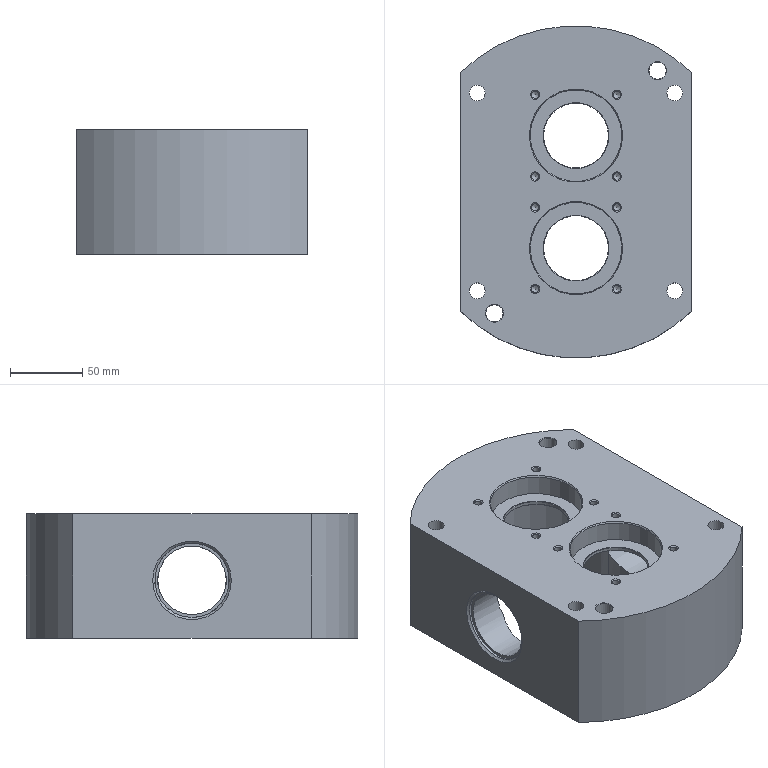NC program | NX | posted with a generic post | part box 160 x 230 x 86 mm
Lines 20253 to 21365 of 21365:
(FLOOR_WALL_1_COPY_COPY , TOOL : D12)
N40480 T12 M6
N40482 G54
N40484 G17 G0 G90 X39.081 Y-47.861 B0. C0. S4000 M3
N40486 G43 Z30. H12
N40488 Z-65.2
N40490 G94 G1 Z-68.2 F500.
N40492 G3 X40.134 Y-48.437 R1.2
N40494 G1 X40.035 Y-48.439 F1000.
N40496 G2 X21.885 Y-45.326 R48.45
N40498 G1 X19.712 Y-44.506
N40500 G3 X19.288 Y-44.506 R0.6
N40502 G1 X17.115 Y-45.326
N40504 G2 X-17.115 Y-45.326 R48.45
N40506 G1 X-19.288 Y-44.506
N40508 G3 X-19.712 Y-44.506 R0.6
N40510 G1 X-21.885 Y-45.326
N40512 G2 X-57.408 Y-44.817 R48.45
N40514 G1 X62.941 Y-42.122
N40516 G3 X71.279 Y-36.131 R48.45
N40518 G1 X-67.423 Y-39.237
N40520 G2 X-73.927 Y-33.578 R48.45
N40522 G1 X76.885 Y-30.201
N40524 G3 X80.912 Y-24.307 R48.45
N40526 G1 X-78.625 Y-27.88
N40528 G2 X-82.089 Y-22.153 R48.45
N40530 G1 X83.805 Y-18.438
N40532 G3 X85.786 Y-12.589 R48.45
N40534 G1 X-84.588 Y-16.405
N40536 G2 X-86.268 Y-10.638 R48.45
N40538 G1 X86.976 Y-6.759
N40540 G3 X87.441 Y-0.944 R48.45
N40542 G1 X-87.206 Y-4.855
N40544 G2 X-87.441 Y0.944 R48.45
N40546 G1 X87.206 Y4.855
N40548 G3 X86.268 Y10.638 R48.45
N40550 G1 X-86.976 Y6.759
N40552 G2 X-85.786 Y12.589 R48.45
N40554 G1 X84.588 Y16.405
N40556 G3 X82.089 Y22.153 R48.45
N40558 G1 X-83.805 Y18.438
N40560 G2 X-80.912 Y24.307 R48.45
N40562 G1 X78.625 Y27.88
N40564 G3 X73.927 Y33.578 R48.45
N40566 G1 X-76.885 Y30.201
N40568 G2 X-71.279 Y36.131 R48.45
N40570 G1 X67.423 Y39.237
N40572 G3 X57.408 Y44.817 R48.45
N40574 G1 X-62.941 Y42.122
N40576 G2 X-40.134 Y48.437 R48.45
N40578 G1 X-40.036 Y48.439
N40580 G2 X-38.983 Y47.862 R1.2
N40582 G1 X-38.997 Y48.461
N40584 G3 X-40.049 Y49.039 R1.2 F500.
N40586 X-21.673 Y-45.887 R-49.05 F1000.
N40588 G1 X-19.5 Y-45.067
N40590 X-17.327 Y-45.887
N40592 G3 X17.327 Y-45.887 R49.05
N40594 G1 X19.5 Y-45.067
N40596 X21.673 Y-45.887
N40598 G3 X21.673 Y45.887 R-49.05
N40600 G1 X19.5 Y45.067
N40602 X17.327 Y45.887
N40604 G3 X-17.327 Y45.887 R49.05
N40606 G1 X-19.5 Y45.067
N40608 X-21.673 Y45.887
N40610 G3 X-40.049 Y49.039 R49.05
N40612 X-41.075 Y48.417 R1.2
N40614 G1 X-42.445 Y45.921
N40616 Z-65.2
N40618 G0 Z30.
N40620 M5
(HOLE_MILLING_1 , TOOL : D10)
N40622 T10 M6
N40624 G54
N40626 G17 G0 G90 X-68.5 Y68.5 B0. C0. S3000 M3
N40628 G43 Z30. H10
N40630 Z0.5
N40632 G94 G3 X-66.75 Y70.25 R1.75 F1600.
N40634 X-68.5 Y72. R1.75
N40636 X-68.5 Y72. Z0.3 I0. J-3.5
N40638 X-68.5 Y72. Z0.1 I0. J-3.5
N40640 X-68.5 Y72. Z-0.1 I0. J-3.5
N40642 X-68.5 Y72. Z-0.3 I0. J-3.5
N40644 X-68.5 Y72. Z-0.5 I0. J-3.5
N40646 X-68.5 Y72. Z-0.7 I0. J-3.5
N40648 X-68.5 Y72. Z-0.9 I0. J-3.5
N40650 X-68.5 Y72. Z-1.1 I0. J-3.5
N40652 X-68.5 Y72. Z-1.3 I0. J-3.5
N40654 X-68.5 Y72. Z-1.5 I0. J-3.5
N40656 X-68.5 Y72. Z-1.7 I0. J-3.5
N40658 X-68.5 Y72. Z-1.9 I0. J-3.5
N40660 X-68.5 Y72. Z-2.1 I0. J-3.5
N40662 X-68.5 Y72. Z-2.3 I0. J-3.5
N40664 X-68.5 Y72. Z-2.5 I0. J-3.5
N40666 X-68.5 Y72. Z-2.7 I0. J-3.5
N40668 X-68.5 Y72. Z-2.9 I0. J-3.5
N40670 X-68.5 Y72. Z-3.1 I0. J-3.5
N40672 X-68.5 Y72. Z-3.3 I0. J-3.5
N40674 X-68.5 Y72. Z-3.5 I0. J-3.5
N40676 X-68.5 Y72. Z-3.7 I0. J-3.5
N40678 X-68.5 Y72. Z-3.9 I0. J-3.5
N40680 X-68.5 Y72. Z-4.1 I0. J-3.5
N40682 X-68.5 Y72. Z-4.3 I0. J-3.5
N40684 X-68.5 Y72. Z-4.5 I0. J-3.5
N40686 X-68.5 Y72. Z-4.7 I0. J-3.5
N40688 X-68.5 Y72. Z-4.9 I0. J-3.5
N40690 X-68.5 Y72. Z-5.1 I0. J-3.5
N40692 X-68.5 Y72. Z-5.3 I0. J-3.5
N40694 X-68.5 Y72. Z-5.5 I0. J-3.5
N40696 X-68.5 Y72. Z-5.7 I0. J-3.5
N40698 X-68.5 Y72. Z-5.9 I0. J-3.5
N40700 X-68.5 Y72. Z-6.1 I0. J-3.5
N40702 X-68.5 Y72. Z-6.3 I0. J-3.5
N40704 X-68.5 Y72. Z-6.5 I0. J-3.5
N40706 X-68.5 Y72. Z-6.7 I0. J-3.5
N40708 X-68.5 Y72. Z-6.9 I0. J-3.5
N40710 X-68.5 Y72. Z-7.1 I0. J-3.5
N40712 X-68.5 Y72. Z-7.3 I0. J-3.5
N40714 X-68.5 Y72. Z-7.5 I0. J-3.5
N40716 X-68.5 Y72. Z-7.7 I0. J-3.5
N40718 X-68.5 Y72. Z-7.9 I0. J-3.5
N40720 X-68.5 Y72. Z-8.1 I0. J-3.5
N40722 X-68.5 Y72. Z-8.3 I0. J-3.5
N40724 X-68.5 Y72. Z-8.5 I0. J-3.5
N40726 X-68.5 Y72. Z-8.7 I0. J-3.5
N40728 X-68.5 Y72. Z-8.9 I0. J-3.5
N40730 X-68.5 Y72. Z-9.1 I0. J-3.5
N40732 X-68.5 Y72. Z-9.3 I0. J-3.5
N40734 X-68.5 Y72. Z-9.5 I0. J-3.5
N40736 X-68.5 Y72. Z-9.7 I0. J-3.5
N40738 X-68.5 Y72. Z-9.9 I0. J-3.5
N40740 X-68.5 Y72. Z-10.1 I0. J-3.5
N40742 X-68.5 Y72. Z-10.3 I0. J-3.5
N40744 X-68.5 Y72. Z-10.5 I0. J-3.5
N40746 X-68.5 Y72. Z-10.7 I0. J-3.5
N40748 X-68.5 Y72. Z-10.9 I0. J-3.5
N40750 X-68.5 Y72. Z-11.1 I0. J-3.5
N40752 X-68.5 Y72. Z-11.3 I0. J-3.5
N40754 X-68.5 Y72. Z-11.5 I0. J-3.5
N40756 X-68.5 Y72. Z-11.7 I0. J-3.5
N40758 X-68.5 Y72. Z-11.9 I0. J-3.5
N40760 X-68.5 Y72. Z-12.1 I0. J-3.5
N40762 X-68.5 Y72. Z-12.3 I0. J-3.5
N40764 X-68.5 Y72. Z-12.5 I0. J-3.5
N40766 X-68.5 Y72. Z-12.7 I0. J-3.5
N40768 X-68.5 Y72. Z-12.9 I0. J-3.5
N40770 X-68.5 Y72. Z-13.1 I0. J-3.5
N40772 X-68.5 Y72. Z-13.3 I0. J-3.5
N40774 X-68.5 Y72. Z-13.5 I0. J-3.5
N40776 X-68.5 Y72. Z-13.7 I0. J-3.5
N40778 X-68.5 Y72. Z-13.9 I0. J-3.5
N40780 X-68.5 Y72. Z-14.1 I0. J-3.5
N40782 X-68.5 Y72. Z-14.3 I0. J-3.5
N40784 X-68.5 Y72. Z-14.5 I0. J-3.5
N40786 X-68.5 Y72. Z-14.7 I0. J-3.5
N40788 X-68.5 Y72. Z-14.9 I0. J-3.5
N40790 X-68.5 Y72. Z-15.1 I0. J-3.5
N40792 X-68.5 Y72. Z-15.3 I0. J-3.5
N40794 X-68.5 Y72. Z-15.5 I0. J-3.5
N40796 X-68.5 Y72. Z-15.7 I0. J-3.5
N40798 X-68.5 Y72. Z-15.9 I0. J-3.5
N40800 X-68.5 Y72. Z-16.1 I0. J-3.5
N40802 X-68.5 Y72. Z-16.3 I0. J-3.5
N40804 X-68.5 Y72. Z-16.5 I0. J-3.5
N40806 X-68.5 Y72. Z-16.7 I0. J-3.5
N40808 X-68.5 Y72. Z-16.9 I0. J-3.5
N40810 X-68.5 Y72. Z-17.1 I0. J-3.5
N40812 X-68.5 Y72. Z-17.3 I0. J-3.5
N40814 X-68.5 Y72. Z-17.5 I0. J-3.5
N40816 X-68.5 Y72. Z-17.7 I0. J-3.5
N40818 X-68.5 Y72. Z-17.9 I0. J-3.5
N40820 X-68.5 Y72. Z-18.1 I0. J-3.5
N40822 X-68.5 Y72. Z-18.3 I0. J-3.5
N40824 X-68.5 Y72. Z-18.5 I0. J-3.5
N40826 X-68.5 Y72. Z-18.7 I0. J-3.5
N40828 X-68.5 Y72. Z-18.9 I0. J-3.5
N40830 X-68.5 Y72. Z-19.1 I0. J-3.5
N40832 X-68.5 Y72. Z-19.3 I0. J-3.5
N40834 X-68.5 Y72. Z-19.5 I0. J-3.5
N40836 X-68.5 Y72. Z-19.7 I0. J-3.5
N40838 X-68.5 Y72. Z-19.9 I0. J-3.5
N40840 X-68.5 Y72. Z-20.1 I0. J-3.5
N40842 X-68.5 Y72. Z-20.3 I0. J-3.5
N40844 X-68.5 Y72. Z-20.5 I0. J-3.5
N40846 X-68.5 Y72. Z-20.7 I0. J-3.5
N40848 X-68.5 Y72. Z-20.9 I0. J-3.5
N40850 X-68.5 Y72. Z-21.1 I0. J-3.5
N40852 X-68.5 Y72. Z-21.3 I0. J-3.5
N40854 X-68.5 Y72. Z-21.5 I0. J-3.5
N40856 X-68.5 Y72. Z-21.7 I0. J-3.5
N40858 X-68.5 Y72. Z-21.9 I0. J-3.5
N40860 X-68.5 Y72. Z-22.1 I0. J-3.5
N40862 X-68.5 Y72. Z-22.3 I0. J-3.5
N40864 X-68.5 Y72. Z-22.5 I0. J-3.5
N40866 X-68.5 Y72. Z-22.7 I0. J-3.5
N40868 X-68.5 Y72. Z-22.9 I0. J-3.5
N40870 X-68.5 Y72. Z-23.1 I0. J-3.5
N40872 X-68.5 Y72. Z-23.3 I0. J-3.5
N40874 X-68.5 Y72. Z-23.5 I0. J-3.5
N40876 X-68.5 Y72. Z-23.7 I0. J-3.5
N40878 X-68.5 Y72. Z-23.9 I0. J-3.5
N40880 X-68.5 Y72. Z-24.1 I0. J-3.5
N40882 X-68.5 Y72. Z-24.3 I0. J-3.5
N40884 X-68.5 Y72. Z-24.5 I0. J-3.5
N40886 X-68.5 Y72. Z-24.7 I0. J-3.5
N40888 X-68.5 Y72. Z-24.9 I0. J-3.5
N40890 X-68.5 Y72. Z-25.1 I0. J-3.5
N40892 X-68.5 Y72. Z-25.3 I0. J-3.5
N40894 X-68.5 Y72. Z-25.5 I0. J-3.5
N40896 X-68.5 Y72. Z-25.7 I0. J-3.5
N40898 X-68.5 Y72. Z-25.9 I0. J-3.5
N40900 X-68.5 Y72. Z-26.1 I0. J-3.5
N40902 X-68.5 Y72. Z-26.3 I0. J-3.5
N40904 X-68.5 Y72. Z-26.5 I0. J-3.5
N40906 X-68.5 Y72. Z-26.7 I0. J-3.5
N40908 X-68.5 Y72. Z-26.9 I0. J-3.5
N40910 X-68.5 Y72. Z-27.1 I0. J-3.5
N40912 X-68.5 Y72. Z-27.3 I0. J-3.5
N40914 X-68.5 Y72. Z-27.5 I0. J-3.5
N40916 X-68.5 Y72. Z-27.7 I0. J-3.5
N40918 X-68.5 Y72. Z-27.9 I0. J-3.5
N40920 X-68.5 Y72. Z-28.1 I0. J-3.5
N40922 X-68.5 Y72. Z-28.3 I0. J-3.5
N40924 X-68.5 Y72. Z-28.5 I0. J-3.5
N40926 X-68.5 Y72. Z-28.7 I0. J-3.5
N40928 X-68.5 Y72. Z-28.9 I0. J-3.5
N40930 X-68.5 Y72. Z-29.1 I0. J-3.5
N40932 X-68.5 Y72. Z-29.3 I0. J-3.5
N40934 X-68.5 Y72. Z-29.5 I0. J-3.5
N40936 X-68.5 Y72. Z-29.7 I0. J-3.5
N40938 X-68.5 Y72. Z-29.9 I0. J-3.5
N40940 X-68.5 Y72. Z-30.1 I0. J-3.5
N40942 X-68.5 Y72. Z-30.3 I0. J-3.5
N40944 X-68.5 Y72. Z-30.5 I0. J-3.5
N40946 X-68.5 Y72. Z-30.7 I0. J-3.5
N40948 X-68.5 Y72. Z-30.9 I0. J-3.5
N40950 X-68.5 Y65. Z-31. I0. J-3.5
N40952 X-65. Y68.5 R3.5
N40954 X-68.5 Y65. R-3.5
N40956 X-66.75 Y66.75 R1.75
N40958 X-68.5 Y68.5 R1.75
N40960 G0 Z30.
N40962 X68.5
N40964 Z0.5
N40966 G3 X70.25 Y70.25 R1.75
N40968 X68.5 Y72. R1.75
N40970 X68.5 Y72. Z0.3 I0. J-3.5
N40972 X68.5 Y72. Z0.1 I0. J-3.5
N40974 X68.5 Y72. Z-0.1 I0. J-3.5
N40976 X68.5 Y72. Z-0.3 I0. J-3.5
N40978 X68.5 Y72. Z-0.5 I0. J-3.5
N40980 X68.5 Y72. Z-0.7 I0. J-3.5
N40982 X68.5 Y72. Z-0.9 I0. J-3.5
N40984 X68.5 Y72. Z-1.1 I0. J-3.5
N40986 X68.5 Y72. Z-1.3 I0. J-3.5
N40988 X68.5 Y72. Z-1.5 I0. J-3.5
N40990 X68.5 Y72. Z-1.7 I0. J-3.5
N40992 X68.5 Y72. Z-1.9 I0. J-3.5
N40994 X68.5 Y72. Z-2.1 I0. J-3.5
N40996 X68.5 Y72. Z-2.3 I0. J-3.5
N40998 X68.5 Y72. Z-2.5 I0. J-3.5
N41000 X68.5 Y72. Z-2.7 I0. J-3.5
N41002 X68.5 Y72. Z-2.9 I0. J-3.5
N41004 X68.5 Y72. Z-3.1 I0. J-3.5
N41006 X68.5 Y72. Z-3.3 I0. J-3.5
N41008 X68.5 Y72. Z-3.5 I0. J-3.5
N41010 X68.5 Y72. Z-3.7 I0. J-3.5
N41012 X68.5 Y72. Z-3.9 I0. J-3.5
N41014 X68.5 Y72. Z-4.1 I0. J-3.5
N41016 X68.5 Y72. Z-4.3 I0. J-3.5
N41018 X68.5 Y72. Z-4.5 I0. J-3.5
N41020 X68.5 Y72. Z-4.7 I0. J-3.5
N41022 X68.5 Y72. Z-4.9 I0. J-3.5
N41024 X68.5 Y72. Z-5.1 I0. J-3.5
N41026 X68.5 Y72. Z-5.3 I0. J-3.5
N41028 X68.5 Y72. Z-5.5 I0. J-3.5
N41030 X68.5 Y72. Z-5.7 I0. J-3.5
N41032 X68.5 Y72. Z-5.9 I0. J-3.5
N41034 X68.5 Y72. Z-6.1 I0. J-3.5
N41036 X68.5 Y72. Z-6.3 I0. J-3.5
N41038 X68.5 Y72. Z-6.5 I0. J-3.5
N41040 X68.5 Y72. Z-6.7 I0. J-3.5
N41042 X68.5 Y72. Z-6.9 I0. J-3.5
N41044 X68.5 Y72. Z-7.1 I0. J-3.5
N41046 X68.5 Y72. Z-7.3 I0. J-3.5
N41048 X68.5 Y72. Z-7.5 I0. J-3.5
N41050 X68.5 Y72. Z-7.7 I0. J-3.5
N41052 X68.5 Y72. Z-7.9 I0. J-3.5
N41054 X68.5 Y72. Z-8.1 I0. J-3.5
N41056 X68.5 Y72. Z-8.3 I0. J-3.5
N41058 X68.5 Y72. Z-8.5 I0. J-3.5
N41060 X68.5 Y72. Z-8.7 I0. J-3.5
N41062 X68.5 Y72. Z-8.9 I0. J-3.5
N41064 X68.5 Y72. Z-9.1 I0. J-3.5
N41066 X68.5 Y72. Z-9.3 I0. J-3.5
N41068 X68.5 Y72. Z-9.5 I0. J-3.5
N41070 X68.5 Y72. Z-9.7 I0. J-3.5
N41072 X68.5 Y72. Z-9.9 I0. J-3.5
N41074 X68.5 Y72. Z-10.1 I0. J-3.5
N41076 X68.5 Y72. Z-10.3 I0. J-3.5
N41078 X68.5 Y72. Z-10.5 I0. J-3.5
N41080 X68.5 Y72. Z-10.7 I0. J-3.5
N41082 X68.5 Y72. Z-10.9 I0. J-3.5
N41084 X68.5 Y72. Z-11.1 I0. J-3.5
N41086 X68.5 Y72. Z-11.3 I0. J-3.5
N41088 X68.5 Y72. Z-11.5 I0. J-3.5
N41090 X68.5 Y72. Z-11.7 I0. J-3.5
N41092 X68.5 Y72. Z-11.9 I0. J-3.5
N41094 X68.5 Y72. Z-12.1 I0. J-3.5
N41096 X68.5 Y72. Z-12.3 I0. J-3.5
N41098 X68.5 Y72. Z-12.5 I0. J-3.5
N41100 X68.5 Y72. Z-12.7 I0. J-3.5
N41102 X68.5 Y72. Z-12.9 I0. J-3.5
N41104 X68.5 Y72. Z-13.1 I0. J-3.5
N41106 X68.5 Y72. Z-13.3 I0. J-3.5
N41108 X68.5 Y72. Z-13.5 I0. J-3.5
N41110 X68.5 Y72. Z-13.7 I0. J-3.5
N41112 X68.5 Y72. Z-13.9 I0. J-3.5
N41114 X68.5 Y72. Z-14.1 I0. J-3.5
N41116 X68.5 Y72. Z-14.3 I0. J-3.5
N41118 X68.5 Y72. Z-14.5 I0. J-3.5
N41120 X68.5 Y72. Z-14.7 I0. J-3.5
N41122 X68.5 Y72. Z-14.9 I0. J-3.5
N41124 X68.5 Y72. Z-15.1 I0. J-3.5
N41126 X68.5 Y72. Z-15.3 I0. J-3.5
N41128 X68.5 Y72. Z-15.5 I0. J-3.5
N41130 X68.5 Y72. Z-15.7 I0. J-3.5
N41132 X68.5 Y72. Z-15.9 I0. J-3.5
N41134 X68.5 Y72. Z-16.1 I0. J-3.5
N41136 X68.5 Y72. Z-16.3 I0. J-3.5
N41138 X68.5 Y72. Z-16.5 I0. J-3.5
N41140 X68.5 Y72. Z-16.7 I0. J-3.5
N41142 X68.5 Y72. Z-16.9 I0. J-3.5
N41144 X68.5 Y72. Z-17.1 I0. J-3.5
N41146 X68.5 Y72. Z-17.3 I0. J-3.5
N41148 X68.5 Y72. Z-17.5 I0. J-3.5
N41150 X68.5 Y72. Z-17.7 I0. J-3.5
N41152 X68.5 Y72. Z-17.9 I0. J-3.5
N41154 X68.5 Y72. Z-18.1 I0. J-3.5
N41156 X68.5 Y72. Z-18.3 I0. J-3.5
N41158 X68.5 Y72. Z-18.5 I0. J-3.5
N41160 X68.5 Y72. Z-18.7 I0. J-3.5
N41162 X68.5 Y72. Z-18.9 I0. J-3.5
N41164 X68.5 Y72. Z-19.1 I0. J-3.5
N41166 X68.5 Y72. Z-19.3 I0. J-3.5
N41168 X68.5 Y72. Z-19.5 I0. J-3.5
N41170 X68.5 Y72. Z-19.7 I0. J-3.5
N41172 X68.5 Y72. Z-19.9 I0. J-3.5
N41174 X68.5 Y72. Z-20.1 I0. J-3.5
N41176 X68.5 Y72. Z-20.3 I0. J-3.5
N41178 X68.5 Y72. Z-20.5 I0. J-3.5
N41180 X68.5 Y72. Z-20.7 I0. J-3.5
N41182 X68.5 Y72. Z-20.9 I0. J-3.5
N41184 X68.5 Y72. Z-21.1 I0. J-3.5
N41186 X68.5 Y72. Z-21.3 I0. J-3.5
N41188 X68.5 Y72. Z-21.5 I0. J-3.5
N41190 X68.5 Y72. Z-21.7 I0. J-3.5
N41192 X68.5 Y72. Z-21.9 I0. J-3.5
N41194 X68.5 Y72. Z-22.1 I0. J-3.5
N41196 X68.5 Y72. Z-22.3 I0. J-3.5
N41198 X68.5 Y72. Z-22.5 I0. J-3.5
N41200 X68.5 Y72. Z-22.7 I0. J-3.5
N41202 X68.5 Y72. Z-22.9 I0. J-3.5
N41204 X68.5 Y72. Z-23.1 I0. J-3.5
N41206 X68.5 Y72. Z-23.3 I0. J-3.5
N41208 X68.5 Y72. Z-23.5 I0. J-3.5
N41210 X68.5 Y72. Z-23.7 I0. J-3.5
N41212 X68.5 Y72. Z-23.9 I0. J-3.5
N41214 X68.5 Y72. Z-24.1 I0. J-3.5
N41216 X68.5 Y72. Z-24.3 I0. J-3.5
N41218 X68.5 Y72. Z-24.5 I0. J-3.5
N41220 X68.5 Y72. Z-24.7 I0. J-3.5
N41222 X68.5 Y72. Z-24.9 I0. J-3.5
N41224 X68.5 Y72. Z-25.1 I0. J-3.5
N41226 X68.5 Y72. Z-25.3 I0. J-3.5
N41228 X68.5 Y72. Z-25.5 I0. J-3.5
N41230 X68.5 Y72. Z-25.7 I0. J-3.5
N41232 X68.5 Y72. Z-25.9 I0. J-3.5
N41234 X68.5 Y72. Z-26.1 I0. J-3.5
N41236 X68.5 Y72. Z-26.3 I0. J-3.5
N41238 X68.5 Y72. Z-26.5 I0. J-3.5
N41240 X68.5 Y72. Z-26.7 I0. J-3.5
N41242 X68.5 Y72. Z-26.9 I0. J-3.5
N41244 X68.5 Y72. Z-27.1 I0. J-3.5
N41246 X68.5 Y72. Z-27.3 I0. J-3.5
N41248 X68.5 Y72. Z-27.5 I0. J-3.5
N41250 X68.5 Y72. Z-27.7 I0. J-3.5
N41252 X68.5 Y72. Z-27.9 I0. J-3.5
N41254 X68.5 Y72. Z-28.1 I0. J-3.5
N41256 X68.5 Y72. Z-28.3 I0. J-3.5
N41258 X68.5 Y72. Z-28.5 I0. J-3.5
N41260 X68.5 Y72. Z-28.7 I0. J-3.5
N41262 X68.5 Y72. Z-28.9 I0. J-3.5
N41264 X68.5 Y72. Z-29.1 I0. J-3.5
N41266 X68.5 Y72. Z-29.3 I0. J-3.5
N41268 X68.5 Y72. Z-29.5 I0. J-3.5
N41270 X68.5 Y72. Z-29.7 I0. J-3.5
N41272 X68.5 Y72. Z-29.9 I0. J-3.5
N41274 X68.5 Y72. Z-30.1 I0. J-3.5
N41276 X68.5 Y72. Z-30.3 I0. J-3.5
N41278 X68.5 Y72. Z-30.5 I0. J-3.5
N41280 X68.5 Y72. Z-30.7 I0. J-3.5
N41282 X68.5 Y72. Z-30.9 I0. J-3.5
N41284 X68.5 Y65. Z-31. I0. J-3.5
N41286 X72. Y68.5 R3.5
N41288 X68.5 Y65. R-3.5
N41290 X70.25 Y66.75 R1.75
N41292 X68.5 Y68.5 R1.75
N41294 G0 Z30.
N41296 Y-68.5
N41298 Z0.5
N41300 G3 X70.25 Y-66.75 R1.75
N41302 X68.5 Y-65. R1.75
N41304 X68.5 Y-65. Z0.3 I0. J-3.5
N41306 X68.5 Y-65. Z0.1 I0. J-3.5
N41308 X68.5 Y-65. Z-0.1 I0. J-3.5
N41310 X68.5 Y-65. Z-0.3 I0. J-3.5
N41312 X68.5 Y-65. Z-0.5 I0. J-3.5
N41314 X68.5 Y-65. Z-0.7 I0. J-3.5
N41316 X68.5 Y-65. Z-0.9 I0. J-3.5
N41318 X68.5 Y-65. Z-1.1 I0. J-3.5
N41320 X68.5 Y-65. Z-1.3 I0. J-3.5
N41322 X68.5 Y-65. Z-1.5 I0. J-3.5
N41324 X68.5 Y-65. Z-1.7 I0. J-3.5
N41326 X68.5 Y-65. Z-1.9 I0. J-3.5
N41328 X68.5 Y-65. Z-2.1 I0. J-3.5
N41330 X68.5 Y-65. Z-2.3 I0. J-3.5
N41332 X68.5 Y-65. Z-2.5 I0. J-3.5
N41334 X68.5 Y-65. Z-2.7 I0. J-3.5
N41336 X68.5 Y-65. Z-2.9 I0. J-3.5
N41338 X68.5 Y-65. Z-3.1 I0. J-3.5
N41340 X68.5 Y-65. Z-3.3 I0. J-3.5
N41342 X68.5 Y-65. Z-3.5 I0. J-3.5
N41344 X68.5 Y-65. Z-3.7 I0. J-3.5
N41346 X68.5 Y-65. Z-3.9 I0. J-3.5
N41348 X68.5 Y-65. Z-4.1 I0. J-3.5
N41350 X68.5 Y-65. Z-4.3 I0. J-3.5
N41352 X68.5 Y-65. Z-4.5 I0. J-3.5
N41354 X68.5 Y-65. Z-4.7 I0. J-3.5
N41356 X68.5 Y-65. Z-4.9 I0. J-3.5
N41358 X68.5 Y-65. Z-5.1 I0. J-3.5
N41360 X68.5 Y-65. Z-5.3 I0. J-3.5
N41362 X68.5 Y-65. Z-5.5 I0. J-3.5
N41364 X68.5 Y-65. Z-5.7 I0. J-3.5
N41366 X68.5 Y-65. Z-5.9 I0. J-3.5
N41368 X68.5 Y-65. Z-6.1 I0. J-3.5
N41370 X68.5 Y-65. Z-6.3 I0. J-3.5
N41372 X68.5 Y-65. Z-6.5 I0. J-3.5
N41374 X68.5 Y-65. Z-6.7 I0. J-3.5
N41376 X68.5 Y-65. Z-6.9 I0. J-3.5
N41378 X68.5 Y-65. Z-7.1 I0. J-3.5
N41380 X68.5 Y-65. Z-7.3 I0. J-3.5
N41382 X68.5 Y-65. Z-7.5 I0. J-3.5
N41384 X68.5 Y-65. Z-7.7 I0. J-3.5
N41386 X68.5 Y-65. Z-7.9 I0. J-3.5
N41388 X68.5 Y-65. Z-8.1 I0. J-3.5
N41390 X68.5 Y-65. Z-8.3 I0. J-3.5
N41392 X68.5 Y-65. Z-8.5 I0. J-3.5
N41394 X68.5 Y-65. Z-8.7 I0. J-3.5
N41396 X68.5 Y-65. Z-8.9 I0. J-3.5
N41398 X68.5 Y-65. Z-9.1 I0. J-3.5
N41400 X68.5 Y-65. Z-9.3 I0. J-3.5
N41402 X68.5 Y-65. Z-9.5 I0. J-3.5
N41404 X68.5 Y-65. Z-9.7 I0. J-3.5
N41406 X68.5 Y-65. Z-9.9 I0. J-3.5
N41408 X68.5 Y-65. Z-10.1 I0. J-3.5
N41410 X68.5 Y-65. Z-10.3 I0. J-3.5
N41412 X68.5 Y-65. Z-10.5 I0. J-3.5
N41414 X68.5 Y-65. Z-10.7 I0. J-3.5
N41416 X68.5 Y-65. Z-10.9 I0. J-3.5
N41418 X68.5 Y-65. Z-11.1 I0. J-3.5
N41420 X68.5 Y-65. Z-11.3 I0. J-3.5
N41422 X68.5 Y-65. Z-11.5 I0. J-3.5
N41424 X68.5 Y-65. Z-11.7 I0. J-3.5
N41426 X68.5 Y-65. Z-11.9 I0. J-3.5
N41428 X68.5 Y-65. Z-12.1 I0. J-3.5
N41430 X68.5 Y-65. Z-12.3 I0. J-3.5
N41432 X68.5 Y-65. Z-12.5 I0. J-3.5
N41434 X68.5 Y-65. Z-12.7 I0. J-3.5
N41436 X68.5 Y-65. Z-12.9 I0. J-3.5
N41438 X68.5 Y-65. Z-13.1 I0. J-3.5
N41440 X68.5 Y-65. Z-13.3 I0. J-3.5
N41442 X68.5 Y-65. Z-13.5 I0. J-3.5
N41444 X68.5 Y-65. Z-13.7 I0. J-3.5
N41446 X68.5 Y-65. Z-13.9 I0. J-3.5
N41448 X68.5 Y-65. Z-14.1 I0. J-3.5
N41450 X68.5 Y-65. Z-14.3 I0. J-3.5
N41452 X68.5 Y-65. Z-14.5 I0. J-3.5
N41454 X68.5 Y-65. Z-14.7 I0. J-3.5
N41456 X68.5 Y-65. Z-14.9 I0. J-3.5
N41458 X68.5 Y-65. Z-15.1 I0. J-3.5
N41460 X68.5 Y-65. Z-15.3 I0. J-3.5
N41462 X68.5 Y-65. Z-15.5 I0. J-3.5
N41464 X68.5 Y-65. Z-15.7 I0. J-3.5
N41466 X68.5 Y-65. Z-15.9 I0. J-3.5
N41468 X68.5 Y-65. Z-16.1 I0. J-3.5
N41470 X68.5 Y-65. Z-16.3 I0. J-3.5
N41472 X68.5 Y-65. Z-16.5 I0. J-3.5
N41474 X68.5 Y-65. Z-16.7 I0. J-3.5
N41476 X68.5 Y-65. Z-16.9 I0. J-3.5
N41478 X68.5 Y-65. Z-17.1 I0. J-3.5
N41480 X68.5 Y-65. Z-17.3 I0. J-3.5
N41482 X68.5 Y-65. Z-17.5 I0. J-3.5
N41484 X68.5 Y-65. Z-17.7 I0. J-3.5
N41486 X68.5 Y-65. Z-17.9 I0. J-3.5
N41488 X68.5 Y-65. Z-18.1 I0. J-3.5
N41490 X68.5 Y-65. Z-18.3 I0. J-3.5
N41492 X68.5 Y-65. Z-18.5 I0. J-3.5
N41494 X68.5 Y-65. Z-18.7 I0. J-3.5
N41496 X68.5 Y-65. Z-18.9 I0. J-3.5
N41498 X68.5 Y-65. Z-19.1 I0. J-3.5
N41500 X68.5 Y-65. Z-19.3 I0. J-3.5
N41502 X68.5 Y-65. Z-19.5 I0. J-3.5
N41504 X68.5 Y-65. Z-19.7 I0. J-3.5
N41506 X68.5 Y-65. Z-19.9 I0. J-3.5
N41508 X68.5 Y-65. Z-20.1 I0. J-3.5
N41510 X68.5 Y-65. Z-20.3 I0. J-3.5
N41512 X68.5 Y-65. Z-20.5 I0. J-3.5
N41514 X68.5 Y-65. Z-20.7 I0. J-3.5
N41516 X68.5 Y-65. Z-20.9 I0. J-3.5
N41518 X68.5 Y-65. Z-21.1 I0. J-3.5
N41520 X68.5 Y-65. Z-21.3 I0. J-3.5
N41522 X68.5 Y-65. Z-21.5 I0. J-3.5
N41524 X68.5 Y-65. Z-21.7 I0. J-3.5
N41526 X68.5 Y-65. Z-21.9 I0. J-3.5
N41528 X68.5 Y-65. Z-22.1 I0. J-3.5
N41530 X68.5 Y-65. Z-22.3 I0. J-3.5
N41532 X68.5 Y-65. Z-22.5 I0. J-3.5
N41534 X68.5 Y-65. Z-22.7 I0. J-3.5
N41536 X68.5 Y-65. Z-22.9 I0. J-3.5
N41538 X68.5 Y-65. Z-23.1 I0. J-3.5
N41540 X68.5 Y-65. Z-23.3 I0. J-3.5
N41542 X68.5 Y-65. Z-23.5 I0. J-3.5
N41544 X68.5 Y-65. Z-23.7 I0. J-3.5
N41546 X68.5 Y-65. Z-23.9 I0. J-3.5
N41548 X68.5 Y-65. Z-24.1 I0. J-3.5
N41550 X68.5 Y-65. Z-24.3 I0. J-3.5
N41552 X68.5 Y-65. Z-24.5 I0. J-3.5
N41554 X68.5 Y-65. Z-24.7 I0. J-3.5
N41556 X68.5 Y-65. Z-24.9 I0. J-3.5
N41558 X68.5 Y-65. Z-25.1 I0. J-3.5
N41560 X68.5 Y-65. Z-25.3 I0. J-3.5
N41562 X68.5 Y-65. Z-25.5 I0. J-3.5
N41564 X68.5 Y-65. Z-25.7 I0. J-3.5
N41566 X68.5 Y-65. Z-25.9 I0. J-3.5
N41568 X68.5 Y-65. Z-26.1 I0. J-3.5
N41570 X68.5 Y-65. Z-26.3 I0. J-3.5
N41572 X68.5 Y-65. Z-26.5 I0. J-3.5
N41574 X68.5 Y-65. Z-26.7 I0. J-3.5
N41576 X68.5 Y-65. Z-26.9 I0. J-3.5
N41578 X68.5 Y-65. Z-27.1 I0. J-3.5
N41580 X68.5 Y-65. Z-27.3 I0. J-3.5
N41582 X68.5 Y-65. Z-27.5 I0. J-3.5
N41584 X68.5 Y-65. Z-27.7 I0. J-3.5
N41586 X68.5 Y-65. Z-27.9 I0. J-3.5
N41588 X68.5 Y-65. Z-28.1 I0. J-3.5
N41590 X68.5 Y-65. Z-28.3 I0. J-3.5
N41592 X68.5 Y-65. Z-28.5 I0. J-3.5
N41594 X68.5 Y-65. Z-28.7 I0. J-3.5
N41596 X68.5 Y-65. Z-28.9 I0. J-3.5
N41598 X68.5 Y-65. Z-29.1 I0. J-3.5
N41600 X68.5 Y-65. Z-29.3 I0. J-3.5
N41602 X68.5 Y-65. Z-29.5 I0. J-3.5
N41604 X68.5 Y-65. Z-29.7 I0. J-3.5
N41606 X68.5 Y-65. Z-29.9 I0. J-3.5
N41608 X68.5 Y-65. Z-30.1 I0. J-3.5
N41610 X68.5 Y-65. Z-30.3 I0. J-3.5
N41612 X68.5 Y-65. Z-30.5 I0. J-3.5
N41614 X68.5 Y-65. Z-30.7 I0. J-3.5
N41616 X68.5 Y-65. Z-30.9 I0. J-3.5
N41618 X68.5 Y-72. Z-31. I0. J-3.5
N41620 X72. Y-68.5 R3.5
N41622 X68.5 Y-72. R-3.5
N41624 X70.25 Y-70.25 R1.75
N41626 X68.5 Y-68.5 R1.75
N41628 G0 Z30.
N41630 X-68.5
N41632 Z0.5
N41634 G3 X-66.75 Y-66.75 R1.75
N41636 X-68.5 Y-65. R1.75
N41638 X-68.5 Y-65. Z0.3 I0. J-3.5
N41640 X-68.5 Y-65. Z0.1 I0. J-3.5
N41642 X-68.5 Y-65. Z-0.1 I0. J-3.5
N41644 X-68.5 Y-65. Z-0.3 I0. J-3.5
N41646 X-68.5 Y-65. Z-0.5 I0. J-3.5
N41648 X-68.5 Y-65. Z-0.7 I0. J-3.5
N41650 X-68.5 Y-65. Z-0.9 I0. J-3.5
N41652 X-68.5 Y-65. Z-1.1 I0. J-3.5
N41654 X-68.5 Y-65. Z-1.3 I0. J-3.5
N41656 X-68.5 Y-65. Z-1.5 I0. J-3.5
N41658 X-68.5 Y-65. Z-1.7 I0. J-3.5
N41660 X-68.5 Y-65. Z-1.9 I0. J-3.5
N41662 X-68.5 Y-65. Z-2.1 I0. J-3.5
N41664 X-68.5 Y-65. Z-2.3 I0. J-3.5
N41666 X-68.5 Y-65. Z-2.5 I0. J-3.5
N41668 X-68.5 Y-65. Z-2.7 I0. J-3.5
N41670 X-68.5 Y-65. Z-2.9 I0. J-3.5
N41672 X-68.5 Y-65. Z-3.1 I0. J-3.5
N41674 X-68.5 Y-65. Z-3.3 I0. J-3.5
N41676 X-68.5 Y-65. Z-3.5 I0. J-3.5
N41678 X-68.5 Y-65. Z-3.7 I0. J-3.5
N41680 X-68.5 Y-65. Z-3.9 I0. J-3.5
N41682 X-68.5 Y-65. Z-4.1 I0. J-3.5
N41684 X-68.5 Y-65. Z-4.3 I0. J-3.5
N41686 X-68.5 Y-65. Z-4.5 I0. J-3.5
N41688 X-68.5 Y-65. Z-4.7 I0. J-3.5
N41690 X-68.5 Y-65. Z-4.9 I0. J-3.5
N41692 X-68.5 Y-65. Z-5.1 I0. J-3.5
N41694 X-68.5 Y-65. Z-5.3 I0. J-3.5
N41696 X-68.5 Y-65. Z-5.5 I0. J-3.5
N41698 X-68.5 Y-65. Z-5.7 I0. J-3.5
N41700 X-68.5 Y-65. Z-5.9 I0. J-3.5
N41702 X-68.5 Y-65. Z-6.1 I0. J-3.5
N41704 X-68.5 Y-65. Z-6.3 I0. J-3.5
N41706 X-68.5 Y-65. Z-6.5 I0. J-3.5
N41708 X-68.5 Y-65. Z-6.7 I0. J-3.5
N41710 X-68.5 Y-65. Z-6.9 I0. J-3.5
N41712 X-68.5 Y-65. Z-7.1 I0. J-3.5
N41714 X-68.5 Y-65. Z-7.3 I0. J-3.5
N41716 X-68.5 Y-65. Z-7.5 I0. J-3.5
N41718 X-68.5 Y-65. Z-7.7 I0. J-3.5
N41720 X-68.5 Y-65. Z-7.9 I0. J-3.5
N41722 X-68.5 Y-65. Z-8.1 I0. J-3.5
N41724 X-68.5 Y-65. Z-8.3 I0. J-3.5
N41726 X-68.5 Y-65. Z-8.5 I0. J-3.5
N41728 X-68.5 Y-65. Z-8.7 I0. J-3.5
N41730 X-68.5 Y-65. Z-8.9 I0. J-3.5
N41732 X-68.5 Y-65. Z-9.1 I0. J-3.5
N41734 X-68.5 Y-65. Z-9.3 I0. J-3.5
N41736 X-68.5 Y-65. Z-9.5 I0. J-3.5
N41738 X-68.5 Y-65. Z-9.7 I0. J-3.5
N41740 X-68.5 Y-65. Z-9.9 I0. J-3.5
N41742 X-68.5 Y-65. Z-10.1 I0. J-3.5
N41744 X-68.5 Y-65. Z-10.3 I0. J-3.5
N41746 X-68.5 Y-65. Z-10.5 I0. J-3.5
N41748 X-68.5 Y-65. Z-10.7 I0. J-3.5
N41750 X-68.5 Y-65. Z-10.9 I0. J-3.5
N41752 X-68.5 Y-65. Z-11.1 I0. J-3.5
N41754 X-68.5 Y-65. Z-11.3 I0. J-3.5
N41756 X-68.5 Y-65. Z-11.5 I0. J-3.5
N41758 X-68.5 Y-65. Z-11.7 I0. J-3.5
N41760 X-68.5 Y-65. Z-11.9 I0. J-3.5
N41762 X-68.5 Y-65. Z-12.1 I0. J-3.5
N41764 X-68.5 Y-65. Z-12.3 I0. J-3.5
N41766 X-68.5 Y-65. Z-12.5 I0. J-3.5
N41768 X-68.5 Y-65. Z-12.7 I0. J-3.5
N41770 X-68.5 Y-65. Z-12.9 I0. J-3.5
N41772 X-68.5 Y-65. Z-13.1 I0. J-3.5
N41774 X-68.5 Y-65. Z-13.3 I0. J-3.5
N41776 X-68.5 Y-65. Z-13.5 I0. J-3.5
N41778 X-68.5 Y-65. Z-13.7 I0. J-3.5
N41780 X-68.5 Y-65. Z-13.9 I0. J-3.5
N41782 X-68.5 Y-65. Z-14.1 I0. J-3.5
N41784 X-68.5 Y-65. Z-14.3 I0. J-3.5
N41786 X-68.5 Y-65. Z-14.5 I0. J-3.5
N41788 X-68.5 Y-65. Z-14.7 I0. J-3.5
N41790 X-68.5 Y-65. Z-14.9 I0. J-3.5
N41792 X-68.5 Y-65. Z-15.1 I0. J-3.5
N41794 X-68.5 Y-65. Z-15.3 I0. J-3.5
N41796 X-68.5 Y-65. Z-15.5 I0. J-3.5
N41798 X-68.5 Y-65. Z-15.7 I0. J-3.5
N41800 X-68.5 Y-65. Z-15.9 I0. J-3.5
N41802 X-68.5 Y-65. Z-16.1 I0. J-3.5
N41804 X-68.5 Y-65. Z-16.3 I0. J-3.5
N41806 X-68.5 Y-65. Z-16.5 I0. J-3.5
N41808 X-68.5 Y-65. Z-16.7 I0. J-3.5
N41810 X-68.5 Y-65. Z-16.9 I0. J-3.5
N41812 X-68.5 Y-65. Z-17.1 I0. J-3.5
N41814 X-68.5 Y-65. Z-17.3 I0. J-3.5
N41816 X-68.5 Y-65. Z-17.5 I0. J-3.5
N41818 X-68.5 Y-65. Z-17.7 I0. J-3.5
N41820 X-68.5 Y-65. Z-17.9 I0. J-3.5
N41822 X-68.5 Y-65. Z-18.1 I0. J-3.5
N41824 X-68.5 Y-65. Z-18.3 I0. J-3.5
N41826 X-68.5 Y-65. Z-18.5 I0. J-3.5
N41828 X-68.5 Y-65. Z-18.7 I0. J-3.5
N41830 X-68.5 Y-65. Z-18.9 I0. J-3.5
N41832 X-68.5 Y-65. Z-19.1 I0. J-3.5
N41834 X-68.5 Y-65. Z-19.3 I0. J-3.5
N41836 X-68.5 Y-65. Z-19.5 I0. J-3.5
N41838 X-68.5 Y-65. Z-19.7 I0. J-3.5
N41840 X-68.5 Y-65. Z-19.9 I0. J-3.5
N41842 X-68.5 Y-65. Z-20.1 I0. J-3.5
N41844 X-68.5 Y-65. Z-20.3 I0. J-3.5
N41846 X-68.5 Y-65. Z-20.5 I0. J-3.5
N41848 X-68.5 Y-65. Z-20.7 I0. J-3.5
N41850 X-68.5 Y-65. Z-20.9 I0. J-3.5
N41852 X-68.5 Y-65. Z-21.1 I0. J-3.5
N41854 X-68.5 Y-65. Z-21.3 I0. J-3.5
N41856 X-68.5 Y-65. Z-21.5 I0. J-3.5
N41858 X-68.5 Y-65. Z-21.7 I0. J-3.5
N41860 X-68.5 Y-65. Z-21.9 I0. J-3.5
N41862 X-68.5 Y-65. Z-22.1 I0. J-3.5
N41864 X-68.5 Y-65. Z-22.3 I0. J-3.5
N41866 X-68.5 Y-65. Z-22.5 I0. J-3.5
N41868 X-68.5 Y-65. Z-22.7 I0. J-3.5
N41870 X-68.5 Y-65. Z-22.9 I0. J-3.5
N41872 X-68.5 Y-65. Z-23.1 I0. J-3.5
N41874 X-68.5 Y-65. Z-23.3 I0. J-3.5
N41876 X-68.5 Y-65. Z-23.5 I0. J-3.5
N41878 X-68.5 Y-65. Z-23.7 I0. J-3.5
N41880 X-68.5 Y-65. Z-23.9 I0. J-3.5
N41882 X-68.5 Y-65. Z-24.1 I0. J-3.5
N41884 X-68.5 Y-65. Z-24.3 I0. J-3.5
N41886 X-68.5 Y-65. Z-24.5 I0. J-3.5
N41888 X-68.5 Y-65. Z-24.7 I0. J-3.5
N41890 X-68.5 Y-65. Z-24.9 I0. J-3.5
N41892 X-68.5 Y-65. Z-25.1 I0. J-3.5
N41894 X-68.5 Y-65. Z-25.3 I0. J-3.5
N41896 X-68.5 Y-65. Z-25.5 I0. J-3.5
N41898 X-68.5 Y-65. Z-25.7 I0. J-3.5
N41900 X-68.5 Y-65. Z-25.9 I0. J-3.5
N41902 X-68.5 Y-65. Z-26.1 I0. J-3.5
N41904 X-68.5 Y-65. Z-26.3 I0. J-3.5
N41906 X-68.5 Y-65. Z-26.5 I0. J-3.5
N41908 X-68.5 Y-65. Z-26.7 I0. J-3.5
N41910 X-68.5 Y-65. Z-26.9 I0. J-3.5
N41912 X-68.5 Y-65. Z-27.1 I0. J-3.5
N41914 X-68.5 Y-65. Z-27.3 I0. J-3.5
N41916 X-68.5 Y-65. Z-27.5 I0. J-3.5
N41918 X-68.5 Y-65. Z-27.7 I0. J-3.5
N41920 X-68.5 Y-65. Z-27.9 I0. J-3.5
N41922 X-68.5 Y-65. Z-28.1 I0. J-3.5
N41924 X-68.5 Y-65. Z-28.3 I0. J-3.5
N41926 X-68.5 Y-65. Z-28.5 I0. J-3.5
N41928 X-68.5 Y-65. Z-28.7 I0. J-3.5
N41930 X-68.5 Y-65. Z-28.9 I0. J-3.5
N41932 X-68.5 Y-65. Z-29.1 I0. J-3.5
N41934 X-68.5 Y-65. Z-29.3 I0. J-3.5
N41936 X-68.5 Y-65. Z-29.5 I0. J-3.5
N41938 X-68.5 Y-65. Z-29.7 I0. J-3.5
N41940 X-68.5 Y-65. Z-29.9 I0. J-3.5
N41942 X-68.5 Y-65. Z-30.1 I0. J-3.5
N41944 X-68.5 Y-65. Z-30.3 I0. J-3.5
N41946 X-68.5 Y-65. Z-30.5 I0. J-3.5
N41948 X-68.5 Y-65. Z-30.7 I0. J-3.5
N41950 X-68.5 Y-65. Z-30.9 I0. J-3.5
N41952 X-68.5 Y-72. Z-31. I0. J-3.5
N41954 X-65. Y-68.5 R3.5
N41956 X-68.5 Y-72. R-3.5
N41958 X-66.75 Y-70.25 R1.75
N41960 X-68.5 Y-68.5 R1.75
N41962 G0 Z30.
N41964 M5
(PLANAR_MILL_COPY_COPY_COPY_1 , TOOL : D6A45)
N41966 T07 M6
N41968 G54
N41970 G17 G0 G90 X-44.638 Y69.324 B0. C0. S7500 M3
N41972 G43 Z30. H7
N41974 Z1.5
N41976 G94 G1 Z-1.5 F1250.
N41978 X-44.234 Y70.243
N41980 G3 X-45. Y70.6 R1.
N41982 X-47.1 Y68.5 R2.1
N41984 X-45. Y70.6 R-2.1
N41986 X-45.766 Y70.243 R1.
N41988 G1 X-45.362 Y69.324
N41990 Z1.5
N41992 G0 Z30.
N41994 X-66.827 Y74.262
N41996 Z1.5
N41998 G1 Z-1.5
N42000 X-67.734 Y75.343
N42002 G3 X-68.5 Y75.7 R1.
N42004 X-75.7 Y68.5 R7.2
N42006 X-68.5 Y75.7 R-7.2
N42008 X-69.266 Y75.343 R1.
N42010 G1 X-70.173 Y74.262
N42012 Z1.5
N42014 G0 Z30.
N42016 X-106.324 Y0.362
N42018 Z1.5
N42020 G1 Z-1.5
N42022 X-107.243 Y0.766
N42024 G3 X-107.6 Y0. R1.
N42026 X-105.5 Y-2.1 R2.1
N42028 X-107.6 Y0. R-2.1
N42030 X-107.243 Y-0.766 R1.
N42032 G1 X-106.324 Y-0.362
N42034 Z1.5
N42036 G0 Z30.
N42038 X-86. Y-59.372
N42040 Z1.5
N42042 G1 Z-1.5
N42044 X-84.766 Y-60.843
N42046 G3 X-84. Y-61.2 R1.
N42048 X-79.3 Y-56.5 R4.7
N42050 X-84. Y-61.2 R-4.7
N42052 X-83.234 Y-60.843 R1.
N42054 G1 X-82. Y-59.372
N42056 Z1.5
N42058 G0 Z30.
N42060 X-70.173 Y-74.262
N42062 Z1.5
N42064 G1 Z-1.5
N42066 X-69.266 Y-75.343
N42068 G3 X-68.5 Y-75.7 R1.
N42070 X-61.3 Y-68.5 R7.2
N42072 X-68.5 Y-75.7 R-7.2
N42074 X-67.734 Y-75.343 R1.
N42076 G1 X-66.827 Y-74.262
N42078 Z1.5
N42080 G0 Z30.
N42082 X-45.362 Y-69.324
N42084 Z1.5
N42086 G1 Z-1.5
N42088 X-45.766 Y-70.243
N42090 G3 X-45. Y-70.6 R1.
N42092 X-42.9 Y-68.5 R2.1
N42094 X-45. Y-70.6 R-2.1
N42096 X-44.234 Y-70.243 R1.
N42098 G1 X-44.638 Y-69.324
N42100 Z1.5
N42102 G0 Z30.
N42104 X-91.679 Y1.491
N42106 Z1.5
N42108 G1 Z-1.5
N42110 X-92.543 Y0.766
N42112 G3 X-92.9 Y0. R1.
N42114 X-20.028 Y-50.451 R53.9
N42116 G2 X-18.972 Y-50.451 R1.5
N42118 G3 X18.972 Y-50.451 R53.9
N42120 G2 X20.028 Y-50.451 R1.5
N42122 G3 X20.028 Y50.451 R-53.9
N42124 G2 X18.972 Y50.451 R1.5
N42126 G3 X-18.972 Y50.451 R53.9
N42128 G2 X-20.028 Y50.451 R1.5
N42130 G3 X-92.9 Y0. R53.9
N42132 X-92.543 Y-0.766 R1.
N42134 G1 X-91.679 Y-1.491
N42136 Z1.5
N42138 G0 Z30.
N42140 X44.638 Y-69.324
N42142 Z1.5
N42144 G1 Z-1.5
N42146 X44.234 Y-70.243
N42148 G3 X45. Y-70.6 R1.
N42150 X47.1 Y-68.5 R2.1
N42152 X45. Y-70.6 R-2.1
N42154 X45.766 Y-70.243 R1.
N42156 G1 X45.362 Y-69.324
N42158 Z1.5
N42160 G0 Z30.
N42162 X66.827 Y-74.262
N42164 Z1.5
N42166 G1 Z-1.5
N42168 X67.734 Y-75.343
N42170 G3 X68.5 Y-75.7 R1.
N42172 X75.7 Y-68.5 R7.2
N42174 X68.5 Y-75.7 R-7.2
N42176 X69.266 Y-75.343 R1.
N42178 G1 X70.173 Y-74.262
N42180 Z1.5
N42182 G0 Z30.
N42184 X106.324 Y-0.362
N42186 Z1.5
N42188 G1 Z-1.5
N42190 X107.243 Y-0.766
N42192 G3 X107.6 Y0. R1.
N42194 X105.5 Y2.1 R2.1
N42196 X107.6 Y0. R-2.1
N42198 X107.243 Y0.766 R1.
N42200 G1 X106.324 Y0.362
N42202 Z1.5
N42204 G0 Z30.
N42206 X86. Y59.372
N42208 Z1.5
N42210 G1 Z-1.5
N42212 X84.766 Y60.843
N42214 G3 X84. Y61.2 R1.
N42216 X79.3 Y56.5 R4.7
N42218 X84. Y61.2 R-4.7
N42220 X83.234 Y60.843 R1.
N42222 G1 X82. Y59.372
N42224 Z1.5
N42226 G0 Z30.
N42228 X70.173 Y74.262
N42230 Z1.5
N42232 G1 Z-1.5
N42234 X69.266 Y75.343
N42236 G3 X68.5 Y75.7 R1.
N42238 X61.3 Y68.5 R7.2
N42240 X68.5 Y75.7 R-7.2
N42242 X67.734 Y75.343 R1.
N42244 G1 X66.827 Y74.262
N42246 Z1.5
N42248 G0 Z30.
N42250 X45.362 Y69.324
N42252 Z1.5
N42254 G1 Z-1.5
N42256 X45.766 Y70.243
N42258 G3 X45. Y70.6 R1.
N42260 X42.9 Y68.5 R2.1
N42262 X45. Y70.6 R-2.1
N42264 X44.234 Y70.243 R1.
N42266 G1 X44.638 Y69.324
N42268 Z1.5
N42270 G0 Z30.
N42272 M5
(刀补12 , TOOL : D12)
N42274 T12 M6
N42276 G54
N42278 G17 G0 G90 X18.416 Y43.162 B0. C0. S5000 M3
N42280 G43 Z30. H12
N42282 Z-15.05
N42284 G94 G1 Z-17.05 F1250.
N42286 G41 X18.417 Y43.262 D12
N42288 X18.123 Y45.052
N42290 G3 X17.363 Y45.981 R1.2
N42292 X16.339 Y46.355 R49.15
N42294 X14.9 Y46.837 R49.15
N42296 G1 X14.891 Y46.827
N42298 X14.793 Y46.86
N42300 Y46.871
N42302 G3 X-14.873 Y46.846 R49.15
N42304 G1 X-14.886 Y46.829
N42306 X-14.897 Y46.811
N42308 X-14.919 Y46.81
N42310 X-14.931 Y46.827
N42312 G3 X-16.03 Y46.462 R49.15
N42314 G1 X-16.033 Y46.453
N42316 X-16.771 Y46.19
N42318 X-16.778 Y46.198
N42320 X-16.874 Y46.163
N42322 X-16.885 Y46.149
N42324 X-16.956 Y46.123
N42326 X-17.019 Y46.108
N42328 X-17.027 Y46.104
N42330 X-17.033 Y46.11
N42332 X-17.03 Y46.118
N42334 G2 X-21.637 Y45.981 R6.05
N42336 G3 X-21.637 Y-45.981 R-49.15
N42338 G2 X-17.16 Y-46.062 R6.05
N42340 G1 X-17.126 Y-46.063
N42342 X-16.034 Y-46.453
N42344 X-16.03 Y-46.463
N42346 G3 X-14.931 Y-46.827 R49.15
N42348 G1 X-14.909 Y-46.812
N42350 X-14.882 Y-46.82
N42352 X-14.872 Y-46.846
N42354 G3 X16.03 Y-46.462 R49.15
N42356 G1 X16.033 Y-46.453
N42358 X16.77 Y-46.19
N42360 X16.777 Y-46.198
N42362 G3 X17.365 Y-45.98 R49.15
N42364 G2 X21.505 Y-45.936 R6.032
N42366 G1 X21.993 Y-46.108
N42368 X22.131 Y-46.157
N42370 X22.144 Y-46.169
N42372 G3 X22.144 Y46.169 R-49.15
N42374 G1 X22.131 Y46.157
N42376 X21.562 Y45.953
N42378 G2 X19.904 Y45.606 R6.118
N42380 X17.363 Y45.981 R6.063
N42382 G3 X16.179 Y45.785 R1.2
N42384 G1 X14.519 Y44.423
N42386 G40
N42388 X14.454 Y44.347
N42390 Z-15.05
N42392 G0 Z30.
N42394 X18.418 Y43.161
N42396 Z-32.1
N42398 G1 Z-34.1
N42400 G41 X18.419 Y43.261
N42402 X18.124 Y45.053
N42404 G3 X17.363 Y45.981 R1.2
N42406 G1 X17.326 Y45.995
N42408 X17.319 Y45.994
N42410 X14.467 Y46.961
N42412 X14.452 Y46.962
N42414 X14.456 Y46.976
N42416 G3 X-14.526 Y46.955 R49.15
N42418 G1 X-14.534 Y46.94
N42420 X-17.022 Y46.098
N42422 X-17.16 Y46.05
N42424 X-17.18 Y46.053
N42426 G2 X-21.637 Y45.981 R6.05
N42428 G3 X-21.637 Y-45.981 R-49.15
N42430 G2 X-17.363 Y-45.981 R6.05
N42432 G1 Y-45.979
N42434 X-17.125 Y-46.06
N42436 X-17.079 Y-46.075
N42438 X-14.99 Y-46.785
N42440 X-14.498 Y-46.951
N42442 X-14.496 Y-46.964
N42444 G3 X14.44 Y-46.981 R49.15
N42446 G1 X14.452 Y-46.966
N42448 X16.956 Y-46.12
N42450 X17.193 Y-46.038
N42452 X17.209 Y-46.039
N42454 X17.367 Y-45.98
N42456 G2 X21.503 Y-45.935 R6.027
N42458 G1 X21.993 Y-46.107
N42460 X22.131 Y-46.157
N42462 X22.144 Y-46.169
N42464 G3 X22.144 Y46.169 R-49.15
N42466 G1 X22.131 Y46.157
N42468 X21.993 Y46.107
N42470 X21.217 Y45.84
N42472 G2 X17.363 Y45.981 R6.06
N42474 G3 X16.179 Y45.786 R1.2
N42476 G1 X14.506 Y44.414
N42478 G40
N42480 X14.441 Y44.338
N42482 Z-32.1
N42484 G0 Z30.
N42486 X18.518 Y43.148
N42488 Z-49.15
N42490 G1 Z-51.15
N42492 G41 X18.516 Y43.248
N42494 X18.153 Y45.075
N42496 G3 X17.362 Y45.978 R1.2
N42498 G1 X14.456 Y46.965
N42500 X14.291 Y47.017
N42502 X14.294 Y47.026
N42504 G3 X-14.455 Y46.976 R49.15
N42506 G1 X-14.452 Y46.962
N42508 X-14.466
N42510 X-17.154 Y46.05
N42512 X-17.208 Y46.031
N42514 X-17.402 Y45.964
N42516 X-17.408
N42518 G2 X-21.637 Y45.981 R6.05
N42520 G3 X-21.637 Y-45.981 R-49.15
N42522 G2 X-17.4 Y-45.967 R6.05
N42524 G1 X-17.094 Y-46.069
N42526 X-14.925 Y-46.807
N42528 X-14.435 Y-46.972
N42530 X-14.422 Y-46.973
N42532 X-14.425 Y-46.986
N42534 G3 X14.44 Y-46.981 R49.15
N42536 G1 X14.437 Y-46.967
N42538 X14.451
N42540 X17.151 Y-46.05
N42542 X17.529 Y-45.92
N42544 G2 X21.503 Y-45.934 R6.031
N42546 G1 X21.993 Y-46.107
N42548 X22.131 Y-46.156
N42550 X22.144 Y-46.169
N42552 G3 X22.144 Y46.169 R-49.15
N42554 G1 X22.131 Y46.156
N42556 X21.993 Y46.107
N42558 X21.218 Y45.84
N42560 G2 X17.402 Y45.964 R6.074
N42562 G1 X17.362 Y45.978
N42564 G3 X16.185 Y45.744 R1.2
N42566 G1 X14.622 Y44.374
N42568 G40
N42570 X14.56 Y44.296
N42572 Z-49.15
N42574 G0 Z30.
N42576 X18.416 Y43.161
N42578 Z-66.2
N42580 G1 Z-68.2
N42582 G41 X18.418 Y43.261
N42584 X18.124 Y45.052
N42586 G3 X17.363 Y45.981 R1.2
N42588 X16.836 Y46.177 R49.15
N42590 G1 X16.814 Y46.163
N42592 X16.736 Y46.19
N42594 X14.871 Y46.82
N42596 X14.658 Y46.892
N42598 X14.651 Y46.915
N42600 G3 X-14.778 Y46.876 R49.15
N42602 G1 X-14.784 Y46.852
N42604 X-16.802 Y46.168
N42606 X-16.813 Y46.161
N42608 X-16.824 Y46.169
N42610 X-16.821 Y46.182
N42612 X-16.955 Y46.133
N42614 X-16.956 Y46.116
N42616 G2 X-17.157 Y46.058 R0.908
N42618 G3 X-17.363 Y45.981 R49.15
N42620 G2 X-21.637 Y45.981 R6.05
N42622 G3 X-21.637 Y-45.981 R-49.15
N42624 G2 X-17.101 Y-46.087 R6.05
N42626 G1 X-17.078 Y-46.073
N42628 X-16.956 Y-46.115
N42630 X-14.784 Y-46.852
N42632 X-14.778 Y-46.876
N42634 G3 X14.778 Y-46.876 R49.15
N42636 G1 X14.784 Y-46.852
N42638 X16.801 Y-46.168
N42640 X16.812 Y-46.161
N42642 X16.823 Y-46.17
N42644 X16.82 Y-46.183
N42646 G3 X17.363 Y-45.981 R49.15
N42648 G2 X21.97 Y-46.118 R6.05
N42650 G1 X21.993 Y-46.107
N42652 X22.131 Y-46.156
N42654 X22.144 Y-46.169
N42656 G3 X22.144 Y46.169 R-49.15
N42658 G1 X22.131 Y46.156
N42660 X21.993 Y46.107
N42662 X21.97 Y46.118
N42664 G2 X17.363 Y45.981 R6.05
N42666 G3 X16.179 Y45.787 R1.2
N42668 G1 X14.501 Y44.412
N42670 G40
N42672 X14.436 Y44.336
N42674 Z-66.2
N42676 G0 Z30.
N42678 M5
N42680 M2